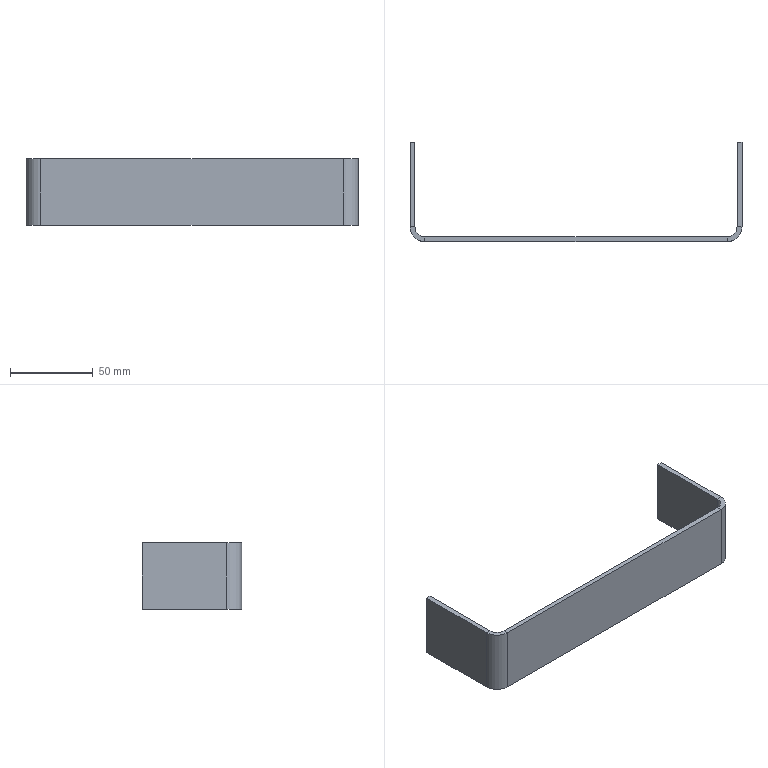Part | SolidWorks | features FlatPattern 1, SMBaseFlange 1, SheetMetal 1 | 1 solid | 22 faces | box 200 x 60 x 40 mm | volume 36907 mm3 | plane 18 | cylinder 4 | commonest cylinder face diameters 12 x2 18 x2
STEP:
#1=CARTESIAN_POINT('',(-135.,-81.,-40.));
#2=VERTEX_POINT('',#1);
#3=CARTESIAN_POINT('',(-138.,-81.,-40.));
#4=VERTEX_POINT('',#3);
#5=CARTESIAN_POINT('',(-135.,-81.,-40.));
#6=DIRECTION('',(-1.,0.,0.));
#7=VECTOR('',#6,1000.);
#8=LINE('',#5,#7);
#9=EDGE_CURVE('',#2,#4,#8,.T.);
#10=ORIENTED_EDGE('',*,*,#9,.F.);
#11=CARTESIAN_POINT('',(-144.,-90.,-40.));
#12=VERTEX_POINT('',#11);
#13=CARTESIAN_POINT('',(-144.,-81.,-40.));
#14=DIRECTION('',(0.,0.,-1.));
#15=DIRECTION('',(1.,0.,0.));
#16=AXIS2_PLACEMENT_3D('',#13,#14,#15);
#17=CIRCLE('',#16,9.);
#18=EDGE_CURVE('',#2,#12,#17,.T.);
#19=ORIENTED_EDGE('',*,*,#18,.T.);
#20=CARTESIAN_POINT('',(-144.,-87.,-40.));
#21=VERTEX_POINT('',#20);
#22=CARTESIAN_POINT('',(-144.,-87.,-40.));
#23=DIRECTION('',(0.,-1.,0.));
#24=VECTOR('',#23,1000.);
#25=LINE('',#22,#24);
#26=EDGE_CURVE('',#21,#12,#25,.T.);
#27=ORIENTED_EDGE('',*,*,#26,.F.);
#28=CARTESIAN_POINT('',(-144.,-81.,-40.));
#29=DIRECTION('',(0.,0.,-1.));
#30=DIRECTION('',(1.,0.,0.));
#31=AXIS2_PLACEMENT_3D('',#28,#29,#30);
#32=CIRCLE('',#31,6.);
#33=EDGE_CURVE('',#4,#21,#32,.T.);
#34=ORIENTED_EDGE('',*,*,#33,.F.);
#35=EDGE_LOOP('',(#10,#19,#27,#34));
#36=FACE_OUTER_BOUND('',#35,.T.);
#37=CARTESIAN_POINT('',(-135.,-81.,-40.));
#38=DIRECTION('',(0.,0.,-1.));
#39=DIRECTION('',(-1.,0.,0.));
#40=AXIS2_PLACEMENT_3D('',#37,#38,#39);
#41=PLANE('',#40);
#42=ADVANCED_FACE('',(#36),#41,.T.);
#43=CARTESIAN_POINT('',(-135.,-30.,-40.));
#44=VERTEX_POINT('',#43);
#45=CARTESIAN_POINT('',(-135.,-30.,-40.));
#46=DIRECTION('',(0.,-1.,0.));
#47=VECTOR('',#46,1000.);
#48=LINE('',#45,#47);
#49=EDGE_CURVE('',#44,#2,#48,.T.);
#50=ORIENTED_EDGE('',*,*,#49,.T.);
#51=ORIENTED_EDGE('',*,*,#9,.T.);
#52=CARTESIAN_POINT('',(-138.,-30.,-40.));
#53=VERTEX_POINT('',#52);
#54=CARTESIAN_POINT('',(-138.,-30.,-40.));
#55=DIRECTION('',(0.,-1.,0.));
#56=VECTOR('',#55,1000.);
#57=LINE('',#54,#56);
#58=EDGE_CURVE('',#53,#4,#57,.T.);
#59=ORIENTED_EDGE('',*,*,#58,.F.);
#60=CARTESIAN_POINT('',(-138.,-30.,-40.));
#61=DIRECTION('',(1.,0.,0.));
#62=VECTOR('',#61,1000.);
#63=LINE('',#60,#62);
#64=EDGE_CURVE('',#53,#44,#63,.T.);
#65=ORIENTED_EDGE('',*,*,#64,.T.);
#66=EDGE_LOOP('',(#50,#51,#59,#65));
#67=FACE_OUTER_BOUND('',#66,.T.);
#68=CARTESIAN_POINT('',(-144.,-87.,-40.));
#69=DIRECTION('',(0.,0.,-1.));
#70=DIRECTION('',(-1.,0.,0.));
#71=AXIS2_PLACEMENT_3D('',#68,#69,#70);
#72=PLANE('',#71);
#73=ADVANCED_FACE('',(#67),#72,.T.);
#74=CARTESIAN_POINT('',(-144.,-90.,0.));
#75=VERTEX_POINT('',#74);
#76=CARTESIAN_POINT('',(-144.,-87.,0.));
#77=VERTEX_POINT('',#76);
#78=CARTESIAN_POINT('',(-144.,-90.,0.));
#79=DIRECTION('',(0.,1.,0.));
#80=VECTOR('',#79,1000.);
#81=LINE('',#78,#80);
#82=EDGE_CURVE('',#75,#77,#81,.T.);
#83=ORIENTED_EDGE('',*,*,#82,.F.);
#84=CARTESIAN_POINT('',(-135.,-81.,0.));
#85=VERTEX_POINT('',#84);
#86=CARTESIAN_POINT('',(-144.,-81.,0.));
#87=DIRECTION('',(0.,0.,-1.));
#88=DIRECTION('',(1.,0.,0.));
#89=AXIS2_PLACEMENT_3D('',#86,#87,#88);
#90=CIRCLE('',#89,9.);
#91=EDGE_CURVE('',#85,#75,#90,.T.);
#92=ORIENTED_EDGE('',*,*,#91,.F.);
#93=CARTESIAN_POINT('',(-138.,-81.,0.));
#94=VERTEX_POINT('',#93);
#95=CARTESIAN_POINT('',(-138.,-81.,0.));
#96=DIRECTION('',(1.,0.,0.));
#97=VECTOR('',#96,1000.);
#98=LINE('',#95,#97);
#99=EDGE_CURVE('',#94,#85,#98,.T.);
#100=ORIENTED_EDGE('',*,*,#99,.F.);
#101=CARTESIAN_POINT('',(-144.,-81.,0.));
#102=DIRECTION('',(0.,0.,-1.));
#103=DIRECTION('',(1.,0.,0.));
#104=AXIS2_PLACEMENT_3D('',#101,#102,#103);
#105=CIRCLE('',#104,6.);
#106=EDGE_CURVE('',#94,#77,#105,.T.);
#107=ORIENTED_EDGE('',*,*,#106,.T.);
#108=EDGE_LOOP('',(#83,#92,#100,#107));
#109=FACE_OUTER_BOUND('',#108,.T.);
#110=CARTESIAN_POINT('',(-144.,-90.,0.));
#111=DIRECTION('',(0.,0.,1.));
#112=DIRECTION('',(1.,0.,0.));
#113=AXIS2_PLACEMENT_3D('',#110,#111,#112);
#114=PLANE('',#113);
#115=ADVANCED_FACE('',(#109),#114,.T.);
#116=CARTESIAN_POINT('',(-326.,-90.,0.));
#117=VERTEX_POINT('',#116);
#118=CARTESIAN_POINT('',(-135.,-90.,0.));
#119=DIRECTION('',(-1.,0.,0.));
#120=VECTOR('',#119,1000.);
#121=LINE('',#118,#120);
#122=EDGE_CURVE('',#75,#117,#121,.T.);
#123=ORIENTED_EDGE('',*,*,#122,.F.);
#124=ORIENTED_EDGE('',*,*,#82,.T.);
#125=CARTESIAN_POINT('',(-326.,-87.,0.));
#126=VERTEX_POINT('',#125);
#127=CARTESIAN_POINT('',(-135.,-87.,0.));
#128=DIRECTION('',(-1.,0.,0.));
#129=VECTOR('',#128,1000.);
#130=LINE('',#127,#129);
#131=EDGE_CURVE('',#77,#126,#130,.T.);
#132=ORIENTED_EDGE('',*,*,#131,.T.);
#133=CARTESIAN_POINT('',(-326.,-87.,0.));
#134=DIRECTION('',(0.,-1.,0.));
#135=VECTOR('',#134,1000.);
#136=LINE('',#133,#135);
#137=EDGE_CURVE('',#126,#117,#136,.T.);
#138=ORIENTED_EDGE('',*,*,#137,.T.);
#139=EDGE_LOOP('',(#123,#124,#132,#138));
#140=FACE_OUTER_BOUND('',#139,.T.);
#141=CARTESIAN_POINT('',(-138.,-81.,0.));
#142=DIRECTION('',(0.,0.,1.));
#143=DIRECTION('',(1.,0.,0.));
#144=AXIS2_PLACEMENT_3D('',#141,#142,#143);
#145=PLANE('',#144);
#146=ADVANCED_FACE('',(#140),#145,.T.);
#147=CARTESIAN_POINT('',(-326.,-90.,-40.));
#148=VERTEX_POINT('',#147);
#149=CARTESIAN_POINT('',(-326.,-87.,-40.));
#150=VERTEX_POINT('',#149);
#151=CARTESIAN_POINT('',(-326.,-90.,-40.));
#152=DIRECTION('',(0.,1.,0.));
#153=VECTOR('',#152,1000.);
#154=LINE('',#151,#153);
#155=EDGE_CURVE('',#148,#150,#154,.T.);
#156=ORIENTED_EDGE('',*,*,#155,.F.);
#157=CARTESIAN_POINT('',(-335.,-81.,-40.));
#158=VERTEX_POINT('',#157);
#159=CARTESIAN_POINT('',(-326.,-81.,-40.));
#160=DIRECTION('',(0.,0.,-1.));
#161=DIRECTION('',(1.,0.,0.));
#162=AXIS2_PLACEMENT_3D('',#159,#160,#161);
#163=CIRCLE('',#162,9.);
#164=EDGE_CURVE('',#148,#158,#163,.T.);
#165=ORIENTED_EDGE('',*,*,#164,.T.);
#166=CARTESIAN_POINT('',(-332.,-81.,-40.));
#167=VERTEX_POINT('',#166);
#168=CARTESIAN_POINT('',(-332.,-81.,-40.));
#169=DIRECTION('',(-1.,0.,0.));
#170=VECTOR('',#169,1000.);
#171=LINE('',#168,#170);
#172=EDGE_CURVE('',#167,#158,#171,.T.);
#173=ORIENTED_EDGE('',*,*,#172,.F.);
#174=CARTESIAN_POINT('',(-326.,-81.,-40.));
#175=DIRECTION('',(0.,0.,-1.));
#176=DIRECTION('',(1.,0.,0.));
#177=AXIS2_PLACEMENT_3D('',#174,#175,#176);
#178=CIRCLE('',#177,6.);
#179=EDGE_CURVE('',#150,#167,#178,.T.);
#180=ORIENTED_EDGE('',*,*,#179,.F.);
#181=EDGE_LOOP('',(#156,#165,#173,#180));
#182=FACE_OUTER_BOUND('',#181,.T.);
#183=CARTESIAN_POINT('',(-326.,-90.,-40.));
#184=DIRECTION('',(0.,0.,-1.));
#185=DIRECTION('',(-1.,0.,0.));
#186=AXIS2_PLACEMENT_3D('',#183,#184,#185);
#187=PLANE('',#186);
#188=ADVANCED_FACE('',(#182),#187,.T.);
#189=CARTESIAN_POINT('',(-135.,-90.,-40.));
#190=DIRECTION('',(-1.,0.,0.));
#191=VECTOR('',#190,1000.);
#192=LINE('',#189,#191);
#193=EDGE_CURVE('',#12,#148,#192,.T.);
#194=ORIENTED_EDGE('',*,*,#193,.T.);
#195=ORIENTED_EDGE('',*,*,#155,.T.);
#196=CARTESIAN_POINT('',(-135.,-87.,-40.));
#197=DIRECTION('',(-1.,0.,0.));
#198=VECTOR('',#197,1000.);
#199=LINE('',#196,#198);
#200=EDGE_CURVE('',#21,#150,#199,.T.);
#201=ORIENTED_EDGE('',*,*,#200,.F.);
#202=ORIENTED_EDGE('',*,*,#26,.T.);
#203=EDGE_LOOP('',(#194,#195,#201,#202));
#204=FACE_OUTER_BOUND('',#203,.T.);
#205=CARTESIAN_POINT('',(-332.,-81.,-40.));
#206=DIRECTION('',(0.,0.,-1.));
#207=DIRECTION('',(-1.,0.,0.));
#208=AXIS2_PLACEMENT_3D('',#205,#206,#207);
#209=PLANE('',#208);
#210=ADVANCED_FACE('',(#204),#209,.T.);
#211=CARTESIAN_POINT('',(-335.,-81.,0.));
#212=VERTEX_POINT('',#211);
#213=CARTESIAN_POINT('',(-332.,-81.,0.));
#214=VERTEX_POINT('',#213);
#215=CARTESIAN_POINT('',(-335.,-81.,0.));
#216=DIRECTION('',(1.,0.,0.));
#217=VECTOR('',#216,1000.);
#218=LINE('',#215,#217);
#219=EDGE_CURVE('',#212,#214,#218,.T.);
#220=ORIENTED_EDGE('',*,*,#219,.F.);
#221=CARTESIAN_POINT('',(-326.,-81.,0.));
#222=DIRECTION('',(0.,0.,-1.));
#223=DIRECTION('',(1.,0.,0.));
#224=AXIS2_PLACEMENT_3D('',#221,#222,#223);
#225=CIRCLE('',#224,9.);
#226=EDGE_CURVE('',#117,#212,#225,.T.);
#227=ORIENTED_EDGE('',*,*,#226,.F.);
#228=ORIENTED_EDGE('',*,*,#137,.F.);
#229=CARTESIAN_POINT('',(-326.,-81.,0.));
#230=DIRECTION('',(0.,0.,-1.));
#231=DIRECTION('',(1.,0.,0.));
#232=AXIS2_PLACEMENT_3D('',#229,#230,#231);
#233=CIRCLE('',#232,6.);
#234=EDGE_CURVE('',#126,#214,#233,.T.);
#235=ORIENTED_EDGE('',*,*,#234,.T.);
#236=EDGE_LOOP('',(#220,#227,#228,#235));
#237=FACE_OUTER_BOUND('',#236,.T.);
#238=CARTESIAN_POINT('',(-335.,-81.,0.));
#239=DIRECTION('',(0.,0.,1.));
#240=DIRECTION('',(1.,0.,0.));
#241=AXIS2_PLACEMENT_3D('',#238,#239,#240);
#242=PLANE('',#241);
#243=ADVANCED_FACE('',(#237),#242,.T.);
#244=CARTESIAN_POINT('',(-335.,-30.,0.));
#245=VERTEX_POINT('',#244);
#246=CARTESIAN_POINT('',(-335.,-90.,0.));
#247=DIRECTION('',(0.,1.,0.));
#248=VECTOR('',#247,1000.);
#249=LINE('',#246,#248);
#250=EDGE_CURVE('',#212,#245,#249,.T.);
#251=ORIENTED_EDGE('',*,*,#250,.F.);
#252=ORIENTED_EDGE('',*,*,#219,.T.);
#253=CARTESIAN_POINT('',(-332.,-30.,0.));
#254=VERTEX_POINT('',#253);
#255=CARTESIAN_POINT('',(-332.,-90.,0.));
#256=DIRECTION('',(0.,1.,0.));
#257=VECTOR('',#256,1000.);
#258=LINE('',#255,#257);
#259=EDGE_CURVE('',#214,#254,#258,.T.);
#260=ORIENTED_EDGE('',*,*,#259,.T.);
#261=CARTESIAN_POINT('',(-335.,-30.,0.));
#262=DIRECTION('',(1.,0.,0.));
#263=VECTOR('',#262,1000.);
#264=LINE('',#261,#263);
#265=EDGE_CURVE('',#245,#254,#264,.T.);
#266=ORIENTED_EDGE('',*,*,#265,.F.);
#267=EDGE_LOOP('',(#251,#252,#260,#266));
#268=FACE_OUTER_BOUND('',#267,.T.);
#269=CARTESIAN_POINT('',(-326.,-87.,0.));
#270=DIRECTION('',(0.,0.,1.));
#271=DIRECTION('',(1.,0.,0.));
#272=AXIS2_PLACEMENT_3D('',#269,#270,#271);
#273=PLANE('',#272);
#274=ADVANCED_FACE('',(#268),#273,.T.);
#275=ORIENTED_EDGE('',*,*,#259,.F.);
#276=CARTESIAN_POINT('',(-332.,-81.,-40.));
#277=DIRECTION('',(0.,0.,1.));
#278=VECTOR('',#277,1000.);
#279=LINE('',#276,#278);
#280=EDGE_CURVE('',#167,#214,#279,.T.);
#281=ORIENTED_EDGE('',*,*,#280,.F.);
#282=CARTESIAN_POINT('',(-332.,-30.,-40.));
#283=VERTEX_POINT('',#282);
#284=CARTESIAN_POINT('',(-332.,-90.,-40.));
#285=DIRECTION('',(0.,1.,0.));
#286=VECTOR('',#285,1000.);
#287=LINE('',#284,#286);
#288=EDGE_CURVE('',#167,#283,#287,.T.);
#289=ORIENTED_EDGE('',*,*,#288,.T.);
#290=CARTESIAN_POINT('',(-332.,-30.,-40.));
#291=DIRECTION('',(0.,0.,1.));
#292=VECTOR('',#291,1000.);
#293=LINE('',#290,#292);
#294=EDGE_CURVE('',#283,#254,#293,.T.);
#295=ORIENTED_EDGE('',*,*,#294,.T.);
#296=EDGE_LOOP('',(#275,#281,#289,#295));
#297=FACE_OUTER_BOUND('',#296,.T.);
#298=CARTESIAN_POINT('',(-332.,-90.,-40.));
#299=DIRECTION('',(1.,0.,0.));
#300=DIRECTION('',(0.,0.,-1.));
#301=AXIS2_PLACEMENT_3D('',#298,#299,#300);
#302=PLANE('',#301);
#303=ADVANCED_FACE('',(#297),#302,.T.);
#304=ORIENTED_EDGE('',*,*,#234,.F.);
#305=CARTESIAN_POINT('',(-326.,-87.,-40.));
#306=DIRECTION('',(0.,0.,1.));
#307=VECTOR('',#306,1000.);
#308=LINE('',#305,#307);
#309=EDGE_CURVE('',#150,#126,#308,.T.);
#310=ORIENTED_EDGE('',*,*,#309,.F.);
#311=ORIENTED_EDGE('',*,*,#179,.T.);
#312=ORIENTED_EDGE('',*,*,#280,.T.);
#313=EDGE_LOOP('',(#304,#310,#311,#312));
#314=FACE_OUTER_BOUND('',#313,.T.);
#315=CARTESIAN_POINT('',(-326.,-81.,-40.));
#316=DIRECTION('',(0.,0.,1.));
#317=DIRECTION('',(1.,0.,0.));
#318=AXIS2_PLACEMENT_3D('',#315,#316,#317);
#319=CYLINDRICAL_SURFACE('',#318,6.);
#320=ADVANCED_FACE('',(#314),#319,.F.);
#321=ORIENTED_EDGE('',*,*,#131,.F.);
#322=CARTESIAN_POINT('',(-144.,-87.,-40.));
#323=DIRECTION('',(0.,0.,1.));
#324=VECTOR('',#323,1000.);
#325=LINE('',#322,#324);
#326=EDGE_CURVE('',#21,#77,#325,.T.);
#327=ORIENTED_EDGE('',*,*,#326,.F.);
#328=ORIENTED_EDGE('',*,*,#200,.T.);
#329=ORIENTED_EDGE('',*,*,#309,.T.);
#330=EDGE_LOOP('',(#321,#327,#328,#329));
#331=FACE_OUTER_BOUND('',#330,.T.);
#332=CARTESIAN_POINT('',(-135.,-87.,-40.));
#333=DIRECTION('',(0.,1.,0.));
#334=DIRECTION('',(-1.,0.,0.));
#335=AXIS2_PLACEMENT_3D('',#332,#333,#334);
#336=PLANE('',#335);
#337=ADVANCED_FACE('',(#331),#336,.T.);
#338=ORIENTED_EDGE('',*,*,#106,.F.);
#339=CARTESIAN_POINT('',(-138.,-81.,-40.));
#340=DIRECTION('',(0.,0.,1.));
#341=VECTOR('',#340,1000.);
#342=LINE('',#339,#341);
#343=EDGE_CURVE('',#4,#94,#342,.T.);
#344=ORIENTED_EDGE('',*,*,#343,.F.);
#345=ORIENTED_EDGE('',*,*,#33,.T.);
#346=ORIENTED_EDGE('',*,*,#326,.T.);
#347=EDGE_LOOP('',(#338,#344,#345,#346));
#348=FACE_OUTER_BOUND('',#347,.T.);
#349=CARTESIAN_POINT('',(-144.,-81.,-40.));
#350=DIRECTION('',(0.,0.,1.));
#351=DIRECTION('',(1.,0.,0.));
#352=AXIS2_PLACEMENT_3D('',#349,#350,#351);
#353=CYLINDRICAL_SURFACE('',#352,6.);
#354=ADVANCED_FACE('',(#348),#353,.F.);
#355=CARTESIAN_POINT('',(-138.,-30.,0.));
#356=VERTEX_POINT('',#355);
#357=CARTESIAN_POINT('',(-138.,-30.,0.));
#358=DIRECTION('',(0.,-1.,0.));
#359=VECTOR('',#358,1000.);
#360=LINE('',#357,#359);
#361=EDGE_CURVE('',#356,#94,#360,.T.);
#362=ORIENTED_EDGE('',*,*,#361,.F.);
#363=CARTESIAN_POINT('',(-138.,-30.,-40.));
#364=DIRECTION('',(0.,0.,1.));
#365=VECTOR('',#364,1000.);
#366=LINE('',#363,#365);
#367=EDGE_CURVE('',#53,#356,#366,.T.);
#368=ORIENTED_EDGE('',*,*,#367,.F.);
#369=ORIENTED_EDGE('',*,*,#58,.T.);
#370=ORIENTED_EDGE('',*,*,#343,.T.);
#371=EDGE_LOOP('',(#362,#368,#369,#370));
#372=FACE_OUTER_BOUND('',#371,.T.);
#373=CARTESIAN_POINT('',(-138.,-30.,-40.));
#374=DIRECTION('',(-1.,0.,0.));
#375=DIRECTION('',(0.,0.,1.));
#376=AXIS2_PLACEMENT_3D('',#373,#374,#375);
#377=PLANE('',#376);
#378=ADVANCED_FACE('',(#372),#377,.T.);
#379=CARTESIAN_POINT('',(-135.,-30.,0.));
#380=VERTEX_POINT('',#379);
#381=CARTESIAN_POINT('',(-138.,-30.,0.));
#382=DIRECTION('',(1.,0.,0.));
#383=VECTOR('',#382,1000.);
#384=LINE('',#381,#383);
#385=EDGE_CURVE('',#356,#380,#384,.T.);
#386=ORIENTED_EDGE('',*,*,#385,.T.);
#387=CARTESIAN_POINT('',(-135.,-30.,-40.));
#388=DIRECTION('',(0.,0.,1.));
#389=VECTOR('',#388,1000.);
#390=LINE('',#387,#389);
#391=EDGE_CURVE('',#44,#380,#390,.T.);
#392=ORIENTED_EDGE('',*,*,#391,.F.);
#393=ORIENTED_EDGE('',*,*,#64,.F.);
#394=ORIENTED_EDGE('',*,*,#367,.T.);
#395=EDGE_LOOP('',(#386,#392,#393,#394));
#396=FACE_OUTER_BOUND('',#395,.T.);
#397=CARTESIAN_POINT('',(-138.,-30.,-40.));
#398=DIRECTION('',(0.,-1.,0.));
#399=DIRECTION('',(0.,0.,-1.));
#400=AXIS2_PLACEMENT_3D('',#397,#398,#399);
#401=PLANE('',#400);
#402=ADVANCED_FACE('',(#396),#401,.F.);
#403=CARTESIAN_POINT('',(-135.,-30.,0.));
#404=DIRECTION('',(0.,-1.,0.));
#405=VECTOR('',#404,1000.);
#406=LINE('',#403,#405);
#407=EDGE_CURVE('',#380,#85,#406,.T.);
#408=ORIENTED_EDGE('',*,*,#407,.T.);
#409=CARTESIAN_POINT('',(-135.,-81.,-40.));
#410=DIRECTION('',(0.,0.,1.));
#411=VECTOR('',#410,1000.);
#412=LINE('',#409,#411);
#413=EDGE_CURVE('',#2,#85,#412,.T.);
#414=ORIENTED_EDGE('',*,*,#413,.F.);
#415=ORIENTED_EDGE('',*,*,#49,.F.);
#416=ORIENTED_EDGE('',*,*,#391,.T.);
#417=EDGE_LOOP('',(#408,#414,#415,#416));
#418=FACE_OUTER_BOUND('',#417,.T.);
#419=CARTESIAN_POINT('',(-135.,-30.,-40.));
#420=DIRECTION('',(-1.,0.,0.));
#421=DIRECTION('',(0.,0.,1.));
#422=AXIS2_PLACEMENT_3D('',#419,#420,#421);
#423=PLANE('',#422);
#424=ADVANCED_FACE('',(#418),#423,.F.);
#425=ORIENTED_EDGE('',*,*,#91,.T.);
#426=CARTESIAN_POINT('',(-144.,-90.,-40.));
#427=DIRECTION('',(0.,0.,1.));
#428=VECTOR('',#427,1000.);
#429=LINE('',#426,#428);
#430=EDGE_CURVE('',#12,#75,#429,.T.);
#431=ORIENTED_EDGE('',*,*,#430,.F.);
#432=ORIENTED_EDGE('',*,*,#18,.F.);
#433=ORIENTED_EDGE('',*,*,#413,.T.);
#434=EDGE_LOOP('',(#425,#431,#432,#433));
#435=FACE_OUTER_BOUND('',#434,.T.);
#436=CARTESIAN_POINT('',(-144.,-81.,-40.));
#437=DIRECTION('',(0.,0.,1.));
#438=DIRECTION('',(1.,0.,0.));
#439=AXIS2_PLACEMENT_3D('',#436,#437,#438);
#440=CYLINDRICAL_SURFACE('',#439,9.);
#441=ADVANCED_FACE('',(#435),#440,.T.);
#442=ORIENTED_EDGE('',*,*,#122,.T.);
#443=CARTESIAN_POINT('',(-326.,-90.,-40.));
#444=DIRECTION('',(0.,0.,1.));
#445=VECTOR('',#444,1000.);
#446=LINE('',#443,#445);
#447=EDGE_CURVE('',#148,#117,#446,.T.);
#448=ORIENTED_EDGE('',*,*,#447,.F.);
#449=ORIENTED_EDGE('',*,*,#193,.F.);
#450=ORIENTED_EDGE('',*,*,#430,.T.);
#451=EDGE_LOOP('',(#442,#448,#449,#450));
#452=FACE_OUTER_BOUND('',#451,.T.);
#453=CARTESIAN_POINT('',(-135.,-90.,-40.));
#454=DIRECTION('',(0.,1.,0.));
#455=DIRECTION('',(-1.,0.,0.));
#456=AXIS2_PLACEMENT_3D('',#453,#454,#455);
#457=PLANE('',#456);
#458=ADVANCED_FACE('',(#452),#457,.F.);
#459=ORIENTED_EDGE('',*,*,#226,.T.);
#460=CARTESIAN_POINT('',(-335.,-81.,-40.));
#461=DIRECTION('',(0.,0.,1.));
#462=VECTOR('',#461,1000.);
#463=LINE('',#460,#462);
#464=EDGE_CURVE('',#158,#212,#463,.T.);
#465=ORIENTED_EDGE('',*,*,#464,.F.);
#466=ORIENTED_EDGE('',*,*,#164,.F.);
#467=ORIENTED_EDGE('',*,*,#447,.T.);
#468=EDGE_LOOP('',(#459,#465,#466,#467));
#469=FACE_OUTER_BOUND('',#468,.T.);
#470=CARTESIAN_POINT('',(-326.,-81.,-40.));
#471=DIRECTION('',(0.,0.,1.));
#472=DIRECTION('',(1.,0.,0.));
#473=AXIS2_PLACEMENT_3D('',#470,#471,#472);
#474=CYLINDRICAL_SURFACE('',#473,9.);
#475=ADVANCED_FACE('',(#469),#474,.T.);
#476=ORIENTED_EDGE('',*,*,#250,.T.);
#477=CARTESIAN_POINT('',(-335.,-30.,-40.));
#478=VERTEX_POINT('',#477);
#479=CARTESIAN_POINT('',(-335.,-30.,-40.));
#480=DIRECTION('',(0.,0.,1.));
#481=VECTOR('',#480,1000.);
#482=LINE('',#479,#481);
#483=EDGE_CURVE('',#478,#245,#482,.T.);
#484=ORIENTED_EDGE('',*,*,#483,.F.);
#485=CARTESIAN_POINT('',(-335.,-90.,-40.));
#486=DIRECTION('',(0.,1.,0.));
#487=VECTOR('',#486,1000.);
#488=LINE('',#485,#487);
#489=EDGE_CURVE('',#158,#478,#488,.T.);
#490=ORIENTED_EDGE('',*,*,#489,.F.);
#491=ORIENTED_EDGE('',*,*,#464,.T.);
#492=EDGE_LOOP('',(#476,#484,#490,#491));
#493=FACE_OUTER_BOUND('',#492,.T.);
#494=CARTESIAN_POINT('',(-335.,-90.,-40.));
#495=DIRECTION('',(1.,0.,0.));
#496=DIRECTION('',(0.,0.,-1.));
#497=AXIS2_PLACEMENT_3D('',#494,#495,#496);
#498=PLANE('',#497);
#499=ADVANCED_FACE('',(#493),#498,.F.);
#500=ORIENTED_EDGE('',*,*,#265,.T.);
#501=ORIENTED_EDGE('',*,*,#294,.F.);
#502=CARTESIAN_POINT('',(-335.,-30.,-40.));
#503=DIRECTION('',(1.,0.,0.));
#504=VECTOR('',#503,1000.);
#505=LINE('',#502,#504);
#506=EDGE_CURVE('',#478,#283,#505,.T.);
#507=ORIENTED_EDGE('',*,*,#506,.F.);
#508=ORIENTED_EDGE('',*,*,#483,.T.);
#509=EDGE_LOOP('',(#500,#501,#507,#508));
#510=FACE_OUTER_BOUND('',#509,.T.);
#511=CARTESIAN_POINT('',(-335.,-30.,-40.));
#512=DIRECTION('',(0.,-1.,0.));
#513=DIRECTION('',(0.,0.,-1.));
#514=AXIS2_PLACEMENT_3D('',#511,#512,#513);
#515=PLANE('',#514);
#516=ADVANCED_FACE('',(#510),#515,.F.);
#517=ORIENTED_EDGE('',*,*,#288,.F.);
#518=ORIENTED_EDGE('',*,*,#172,.T.);
#519=ORIENTED_EDGE('',*,*,#489,.T.);
#520=ORIENTED_EDGE('',*,*,#506,.T.);
#521=EDGE_LOOP('',(#517,#518,#519,#520));
#522=FACE_OUTER_BOUND('',#521,.T.);
#523=CARTESIAN_POINT('',(-326.,-81.,-40.));
#524=DIRECTION('',(0.,0.,1.));
#525=DIRECTION('',(1.,0.,0.));
#526=AXIS2_PLACEMENT_3D('',#523,#524,#525);
#527=PLANE('',#526);
#528=ADVANCED_FACE('',(#522),#527,.F.);
#529=ORIENTED_EDGE('',*,*,#361,.T.);
#530=ORIENTED_EDGE('',*,*,#99,.T.);
#531=ORIENTED_EDGE('',*,*,#407,.F.);
#532=ORIENTED_EDGE('',*,*,#385,.F.);
#533=EDGE_LOOP('',(#529,#530,#531,#532));
#534=FACE_OUTER_BOUND('',#533,.T.);
#535=CARTESIAN_POINT('',(-326.,-81.,0.));
#536=DIRECTION('',(0.,0.,1.));
#537=DIRECTION('',(1.,0.,0.));
#538=AXIS2_PLACEMENT_3D('',#535,#536,#537);
#539=PLANE('',#538);
#540=ADVANCED_FACE('',(#534),#539,.T.);
#541=CLOSED_SHELL('',(#42,#73,#115,#146,#188,#210,#243,#274,#303,#320,#337,#354,#378,#402,#424,#441,#458,#475,#499,#516,#528,#540));
#542=MANIFOLD_SOLID_BREP('',#541);
#543=CARTESIAN_POINT('',(0.,0.,0.));
#544=DIRECTION('',(0.,0.,1.));
#545=DIRECTION('',(1.,0.,0.));
#546=AXIS2_PLACEMENT_3D('',#543,#544,#545);
#547=(LENGTH_UNIT()NAMED_UNIT(*)SI_UNIT(.MILLI.,.METRE.));
#548=UNCERTAINTY_MEASURE_WITH_UNIT(LENGTH_MEASURE(0.00001),#547,'','');
#549=(NAMED_UNIT(*)PLANE_ANGLE_UNIT()SI_UNIT($,.RADIAN.));
#550=(NAMED_UNIT(*)SI_UNIT($,.STERADIAN.)SOLID_ANGLE_UNIT());
#551=(GEOMETRIC_REPRESENTATION_CONTEXT(3)GLOBAL_UNCERTAINTY_ASSIGNED_CONTEXT((#548))GLOBAL_UNIT_ASSIGNED_CONTEXT((#547,#549,#550))REPRESENTATION_CONTEXT('',''));
#552=ADVANCED_BREP_SHAPE_REPRESENTATION('',(#542,#546),#551);